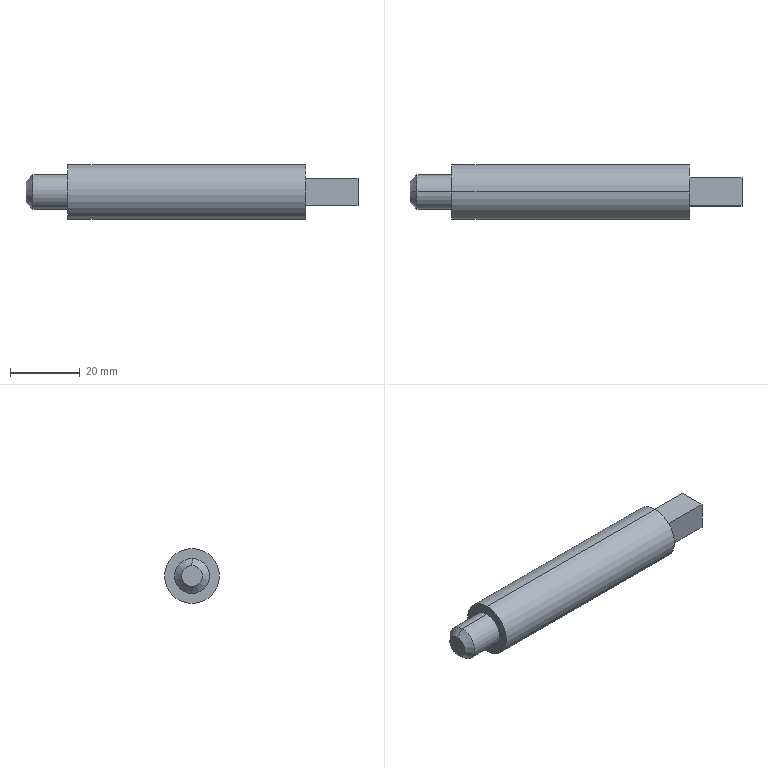Part | SolidWorks | features Chamfer 1, ICE 1, Revolution 1 | 1 solid | 14 faces | box 95 x 15.69 x 15.69 mm | volume 14996 mm3 | plane 8 | cylinder 4 | cone 2 | commonest cylinder face diameters 10 x2 15.69 x2
STEP:
#1=CARTESIAN_POINT('',(0.,0.,3.));
#2=VERTEX_POINT('',#1);
#3=CARTESIAN_POINT('',(0.,0.,-3.));
#4=VERTEX_POINT('',#3);
#5=CARTESIAN_POINT('',(0.,0.,0.));
#6=DIRECTION('',(-1.,0.,0.));
#7=DIRECTION('',(0.,0.,-1.));
#8=AXIS2_PLACEMENT_3D('',#5,#6,#7);
#9=CIRCLE('',#8,3.);
#10=EDGE_CURVE('',#2,#4,#9,.T.);
#11=ORIENTED_EDGE('',*,*,#10,.F.);
#12=CARTESIAN_POINT('',(2.,0.,5.));
#13=VERTEX_POINT('',#12);
#14=CARTESIAN_POINT('',(0.,0.,3.));
#15=DIRECTION('',(0.7071,0.,0.7071));
#16=VECTOR('',#15,1000.);
#17=LINE('',#14,#16);
#18=EDGE_CURVE('',#2,#13,#17,.T.);
#19=ORIENTED_EDGE('',*,*,#18,.T.);
#20=CARTESIAN_POINT('',(2.,0.,-5.));
#21=VERTEX_POINT('',#20);
#22=CARTESIAN_POINT('',(2.,0.,0.));
#23=DIRECTION('',(1.,0.,0.));
#24=DIRECTION('',(0.,0.,-1.));
#25=AXIS2_PLACEMENT_3D('',#22,#23,#24);
#26=CIRCLE('',#25,5.);
#27=EDGE_CURVE('',#21,#13,#26,.T.);
#28=ORIENTED_EDGE('',*,*,#27,.F.);
#29=CARTESIAN_POINT('',(0.,0.,-3.));
#30=DIRECTION('',(0.7071,0.,-0.7071));
#31=VECTOR('',#30,1000.);
#32=LINE('',#29,#31);
#33=EDGE_CURVE('',#4,#21,#32,.T.);
#34=ORIENTED_EDGE('',*,*,#33,.F.);
#35=EDGE_LOOP('',(#11,#19,#28,#34));
#36=FACE_OUTER_BOUND('',#35,.T.);
#37=CARTESIAN_POINT('',(0.,0.,0.));
#38=DIRECTION('',(1.,0.,0.));
#39=DIRECTION('',(0.,0.,-1.));
#40=AXIS2_PLACEMENT_3D('',#37,#38,#39);
#41=CONICAL_SURFACE('',#40,3.,0.7854);
#42=ADVANCED_FACE('',(#36),#41,.T.);
#43=CARTESIAN_POINT('',(80.,0.,7.845));
#44=VERTEX_POINT('',#43);
#45=CARTESIAN_POINT('',(80.,0.,-7.845));
#46=VERTEX_POINT('',#45);
#47=CARTESIAN_POINT('',(80.,0.,0.));
#48=DIRECTION('',(-1.,0.,0.));
#49=DIRECTION('',(0.,0.,1.));
#50=AXIS2_PLACEMENT_3D('',#47,#48,#49);
#51=CIRCLE('',#50,7.845);
#52=EDGE_CURVE('',#44,#46,#51,.T.);
#53=ORIENTED_EDGE('',*,*,#52,.T.);
#54=CARTESIAN_POINT('',(12.,0.,-7.845));
#55=VERTEX_POINT('',#54);
#56=CARTESIAN_POINT('',(0.,0.,-7.845));
#57=DIRECTION('',(-1.,0.,0.));
#58=VECTOR('',#57,1000.);
#59=LINE('',#56,#58);
#60=EDGE_CURVE('',#46,#55,#59,.T.);
#61=ORIENTED_EDGE('',*,*,#60,.T.);
#62=CARTESIAN_POINT('',(12.,0.,7.845));
#63=VERTEX_POINT('',#62);
#64=CARTESIAN_POINT('',(12.,0.,0.));
#65=DIRECTION('',(-1.,0.,0.));
#66=DIRECTION('',(0.,0.,1.));
#67=AXIS2_PLACEMENT_3D('',#64,#65,#66);
#68=CIRCLE('',#67,7.845);
#69=EDGE_CURVE('',#63,#55,#68,.T.);
#70=ORIENTED_EDGE('',*,*,#69,.F.);
#71=CARTESIAN_POINT('',(0.,0.,7.845));
#72=DIRECTION('',(-1.,0.,0.));
#73=VECTOR('',#72,1000.);
#74=LINE('',#71,#73);
#75=EDGE_CURVE('',#44,#63,#74,.T.);
#76=ORIENTED_EDGE('',*,*,#75,.F.);
#77=EDGE_LOOP('',(#53,#61,#70,#76));
#78=FACE_OUTER_BOUND('',#77,.T.);
#79=CARTESIAN_POINT('',(0.,0.,0.));
#80=DIRECTION('',(-1.,0.,0.));
#81=DIRECTION('',(0.,0.,1.));
#82=AXIS2_PLACEMENT_3D('',#79,#80,#81);
#83=CYLINDRICAL_SURFACE('',#82,7.845);
#84=ADVANCED_FACE('',(#78),#83,.T.);
#85=CARTESIAN_POINT('',(12.,0.,5.));
#86=VERTEX_POINT('',#85);
#87=CARTESIAN_POINT('',(12.,0.,-5.));
#88=VERTEX_POINT('',#87);
#89=CARTESIAN_POINT('',(12.,0.,0.));
#90=DIRECTION('',(-1.,0.,0.));
#91=DIRECTION('',(0.,0.,1.));
#92=AXIS2_PLACEMENT_3D('',#89,#90,#91);
#93=CIRCLE('',#92,5.);
#94=EDGE_CURVE('',#86,#88,#93,.T.);
#95=ORIENTED_EDGE('',*,*,#94,.T.);
#96=CARTESIAN_POINT('',(0.,0.,-5.));
#97=DIRECTION('',(-1.,0.,0.));
#98=VECTOR('',#97,1000.);
#99=LINE('',#96,#98);
#100=EDGE_CURVE('',#88,#21,#99,.T.);
#101=ORIENTED_EDGE('',*,*,#100,.T.);
#102=ORIENTED_EDGE('',*,*,#27,.T.);
#103=CARTESIAN_POINT('',(0.,0.,5.));
#104=DIRECTION('',(-1.,0.,0.));
#105=VECTOR('',#104,1000.);
#106=LINE('',#103,#105);
#107=EDGE_CURVE('',#86,#13,#106,.T.);
#108=ORIENTED_EDGE('',*,*,#107,.F.);
#109=EDGE_LOOP('',(#95,#101,#102,#108));
#110=FACE_OUTER_BOUND('',#109,.T.);
#111=CARTESIAN_POINT('',(0.,0.,0.));
#112=DIRECTION('',(-1.,0.,0.));
#113=DIRECTION('',(0.,0.,1.));
#114=AXIS2_PLACEMENT_3D('',#111,#112,#113);
#115=CYLINDRICAL_SURFACE('',#114,5.);
#116=ADVANCED_FACE('',(#110),#115,.T.);
#117=ORIENTED_EDGE('',*,*,#52,.F.);
#118=CARTESIAN_POINT('',(80.,0.,0.));
#119=DIRECTION('',(-1.,0.,0.));
#120=DIRECTION('',(0.,0.,1.));
#121=AXIS2_PLACEMENT_3D('',#118,#119,#120);
#122=CIRCLE('',#121,7.845);
#123=EDGE_CURVE('',#46,#44,#122,.T.);
#124=ORIENTED_EDGE('',*,*,#123,.F.);
#125=EDGE_LOOP('',(#117,#124));
#126=FACE_OUTER_BOUND('',#125,.T.);
#127=CARTESIAN_POINT('',(80.,-4.,-4.));
#128=VERTEX_POINT('',#127);
#129=CARTESIAN_POINT('',(80.,4.,-4.));
#130=VERTEX_POINT('',#129);
#131=CARTESIAN_POINT('',(80.,-4.,-4.));
#132=DIRECTION('',(0.,1.,0.));
#133=VECTOR('',#132,1000.);
#134=LINE('',#131,#133);
#135=EDGE_CURVE('',#128,#130,#134,.T.);
#136=ORIENTED_EDGE('',*,*,#135,.F.);
#137=CARTESIAN_POINT('',(80.,-4.,4.));
#138=VERTEX_POINT('',#137);
#139=CARTESIAN_POINT('',(80.,-4.,4.));
#140=DIRECTION('',(0.,0.,-1.));
#141=VECTOR('',#140,1000.);
#142=LINE('',#139,#141);
#143=EDGE_CURVE('',#138,#128,#142,.T.);
#144=ORIENTED_EDGE('',*,*,#143,.F.);
#145=CARTESIAN_POINT('',(80.,4.,4.));
#146=VERTEX_POINT('',#145);
#147=CARTESIAN_POINT('',(80.,-4.,4.));
#148=DIRECTION('',(0.,-1.,0.));
#149=VECTOR('',#148,1000.);
#150=LINE('',#147,#149);
#151=EDGE_CURVE('',#146,#138,#150,.T.);
#152=ORIENTED_EDGE('',*,*,#151,.F.);
#153=CARTESIAN_POINT('',(80.,4.,4.));
#154=DIRECTION('',(0.,0.,1.));
#155=VECTOR('',#154,1000.);
#156=LINE('',#153,#155);
#157=EDGE_CURVE('',#130,#146,#156,.T.);
#158=ORIENTED_EDGE('',*,*,#157,.F.);
#159=EDGE_LOOP('',(#136,#144,#152,#158));
#160=FACE_BOUND('',#159,.T.);
#161=CARTESIAN_POINT('',(80.,7.845,0.));
#162=DIRECTION('',(-1.,0.,0.));
#163=DIRECTION('',(0.,0.,1.));
#164=AXIS2_PLACEMENT_3D('',#161,#162,#163);
#165=PLANE('',#164);
#166=ADVANCED_FACE('',(#126,#160),#165,.F.);
#167=CARTESIAN_POINT('',(0.,0.,0.));
#168=DIRECTION('',(-1.,0.,0.));
#169=DIRECTION('',(0.,0.,-1.));
#170=AXIS2_PLACEMENT_3D('',#167,#168,#169);
#171=CIRCLE('',#170,3.);
#172=EDGE_CURVE('',#4,#2,#171,.T.);
#173=ORIENTED_EDGE('',*,*,#172,.T.);
#174=ORIENTED_EDGE('',*,*,#10,.T.);
#175=EDGE_LOOP('',(#173,#174));
#176=FACE_OUTER_BOUND('',#175,.T.);
#177=CARTESIAN_POINT('',(0.,0.,0.));
#178=DIRECTION('',(1.,0.,0.));
#179=DIRECTION('',(0.,0.,-1.));
#180=AXIS2_PLACEMENT_3D('',#177,#178,#179);
#181=PLANE('',#180);
#182=ADVANCED_FACE('',(#176),#181,.F.);
#183=ORIENTED_EDGE('',*,*,#100,.F.);
#184=CARTESIAN_POINT('',(12.,0.,0.));
#185=DIRECTION('',(-1.,0.,0.));
#186=DIRECTION('',(0.,0.,1.));
#187=AXIS2_PLACEMENT_3D('',#184,#185,#186);
#188=CIRCLE('',#187,5.);
#189=EDGE_CURVE('',#88,#86,#188,.T.);
#190=ORIENTED_EDGE('',*,*,#189,.T.);
#191=ORIENTED_EDGE('',*,*,#107,.T.);
#192=CARTESIAN_POINT('',(2.,0.,0.));
#193=DIRECTION('',(1.,0.,0.));
#194=DIRECTION('',(0.,0.,-1.));
#195=AXIS2_PLACEMENT_3D('',#192,#193,#194);
#196=CIRCLE('',#195,5.);
#197=EDGE_CURVE('',#13,#21,#196,.T.);
#198=ORIENTED_EDGE('',*,*,#197,.T.);
#199=EDGE_LOOP('',(#183,#190,#191,#198));
#200=FACE_OUTER_BOUND('',#199,.T.);
#201=CARTESIAN_POINT('',(0.,0.,0.));
#202=DIRECTION('',(-1.,0.,0.));
#203=DIRECTION('',(0.,0.,1.));
#204=AXIS2_PLACEMENT_3D('',#201,#202,#203);
#205=CYLINDRICAL_SURFACE('',#204,5.);
#206=ADVANCED_FACE('',(#200),#205,.T.);
#207=ORIENTED_EDGE('',*,*,#94,.F.);
#208=ORIENTED_EDGE('',*,*,#189,.F.);
#209=EDGE_LOOP('',(#207,#208));
#210=FACE_BOUND('',#209,.T.);
#211=ORIENTED_EDGE('',*,*,#69,.T.);
#212=CARTESIAN_POINT('',(12.,0.,0.));
#213=DIRECTION('',(-1.,0.,0.));
#214=DIRECTION('',(0.,0.,1.));
#215=AXIS2_PLACEMENT_3D('',#212,#213,#214);
#216=CIRCLE('',#215,7.845);
#217=EDGE_CURVE('',#55,#63,#216,.T.);
#218=ORIENTED_EDGE('',*,*,#217,.T.);
#219=EDGE_LOOP('',(#211,#218));
#220=FACE_OUTER_BOUND('',#219,.T.);
#221=CARTESIAN_POINT('',(12.,5.,0.));
#222=DIRECTION('',(1.,0.,0.));
#223=DIRECTION('',(0.,0.,-1.));
#224=AXIS2_PLACEMENT_3D('',#221,#222,#223);
#225=PLANE('',#224);
#226=ADVANCED_FACE('',(#210,#220),#225,.F.);
#227=ORIENTED_EDGE('',*,*,#60,.F.);
#228=ORIENTED_EDGE('',*,*,#123,.T.);
#229=ORIENTED_EDGE('',*,*,#75,.T.);
#230=ORIENTED_EDGE('',*,*,#217,.F.);
#231=EDGE_LOOP('',(#227,#228,#229,#230));
#232=FACE_OUTER_BOUND('',#231,.T.);
#233=CARTESIAN_POINT('',(0.,0.,0.));
#234=DIRECTION('',(-1.,0.,0.));
#235=DIRECTION('',(0.,0.,1.));
#236=AXIS2_PLACEMENT_3D('',#233,#234,#235);
#237=CYLINDRICAL_SURFACE('',#236,7.845);
#238=ADVANCED_FACE('',(#232),#237,.T.);
#239=ORIENTED_EDGE('',*,*,#135,.T.);
#240=CARTESIAN_POINT('',(95.,4.,-4.));
#241=VERTEX_POINT('',#240);
#242=CARTESIAN_POINT('',(95.,4.,-4.));
#243=DIRECTION('',(-1.,0.,0.));
#244=VECTOR('',#243,1000.);
#245=LINE('',#242,#244);
#246=EDGE_CURVE('',#241,#130,#245,.T.);
#247=ORIENTED_EDGE('',*,*,#246,.F.);
#248=CARTESIAN_POINT('',(95.,-4.,-4.));
#249=VERTEX_POINT('',#248);
#250=CARTESIAN_POINT('',(95.,-4.,-4.));
#251=DIRECTION('',(0.,1.,0.));
#252=VECTOR('',#251,1000.);
#253=LINE('',#250,#252);
#254=EDGE_CURVE('',#249,#241,#253,.T.);
#255=ORIENTED_EDGE('',*,*,#254,.F.);
#256=CARTESIAN_POINT('',(95.,-4.,-4.));
#257=DIRECTION('',(-1.,0.,0.));
#258=VECTOR('',#257,1000.);
#259=LINE('',#256,#258);
#260=EDGE_CURVE('',#249,#128,#259,.T.);
#261=ORIENTED_EDGE('',*,*,#260,.T.);
#262=EDGE_LOOP('',(#239,#247,#255,#261));
#263=FACE_OUTER_BOUND('',#262,.T.);
#264=CARTESIAN_POINT('',(95.,-4.,-4.));
#265=DIRECTION('',(0.,0.,1.));
#266=DIRECTION('',(1.,0.,0.));
#267=AXIS2_PLACEMENT_3D('',#264,#265,#266);
#268=PLANE('',#267);
#269=ADVANCED_FACE('',(#263),#268,.F.);
#270=ORIENTED_EDGE('',*,*,#157,.T.);
#271=CARTESIAN_POINT('',(95.,4.,4.));
#272=VERTEX_POINT('',#271);
#273=CARTESIAN_POINT('',(95.,4.,4.));
#274=DIRECTION('',(-1.,0.,0.));
#275=VECTOR('',#274,1000.);
#276=LINE('',#273,#275);
#277=EDGE_CURVE('',#272,#146,#276,.T.);
#278=ORIENTED_EDGE('',*,*,#277,.F.);
#279=CARTESIAN_POINT('',(95.,4.,4.));
#280=DIRECTION('',(0.,0.,1.));
#281=VECTOR('',#280,1000.);
#282=LINE('',#279,#281);
#283=EDGE_CURVE('',#241,#272,#282,.T.);
#284=ORIENTED_EDGE('',*,*,#283,.F.);
#285=ORIENTED_EDGE('',*,*,#246,.T.);
#286=EDGE_LOOP('',(#270,#278,#284,#285));
#287=FACE_OUTER_BOUND('',#286,.T.);
#288=CARTESIAN_POINT('',(95.,4.,4.));
#289=DIRECTION('',(0.,-1.,0.));
#290=DIRECTION('',(0.,0.,-1.));
#291=AXIS2_PLACEMENT_3D('',#288,#289,#290);
#292=PLANE('',#291);
#293=ADVANCED_FACE('',(#287),#292,.F.);
#294=ORIENTED_EDGE('',*,*,#151,.T.);
#295=CARTESIAN_POINT('',(95.,-4.,4.));
#296=VERTEX_POINT('',#295);
#297=CARTESIAN_POINT('',(95.,-4.,4.));
#298=DIRECTION('',(-1.,0.,0.));
#299=VECTOR('',#298,1000.);
#300=LINE('',#297,#299);
#301=EDGE_CURVE('',#296,#138,#300,.T.);
#302=ORIENTED_EDGE('',*,*,#301,.F.);
#303=CARTESIAN_POINT('',(95.,-4.,4.));
#304=DIRECTION('',(0.,-1.,0.));
#305=VECTOR('',#304,1000.);
#306=LINE('',#303,#305);
#307=EDGE_CURVE('',#272,#296,#306,.T.);
#308=ORIENTED_EDGE('',*,*,#307,.F.);
#309=ORIENTED_EDGE('',*,*,#277,.T.);
#310=EDGE_LOOP('',(#294,#302,#308,#309));
#311=FACE_OUTER_BOUND('',#310,.T.);
#312=CARTESIAN_POINT('',(95.,-4.,4.));
#313=DIRECTION('',(0.,0.,-1.));
#314=DIRECTION('',(-1.,0.,0.));
#315=AXIS2_PLACEMENT_3D('',#312,#313,#314);
#316=PLANE('',#315);
#317=ADVANCED_FACE('',(#311),#316,.F.);
#318=ORIENTED_EDGE('',*,*,#143,.T.);
#319=ORIENTED_EDGE('',*,*,#260,.F.);
#320=CARTESIAN_POINT('',(95.,-4.,4.));
#321=DIRECTION('',(0.,0.,-1.));
#322=VECTOR('',#321,1000.);
#323=LINE('',#320,#322);
#324=EDGE_CURVE('',#296,#249,#323,.T.);
#325=ORIENTED_EDGE('',*,*,#324,.F.);
#326=ORIENTED_EDGE('',*,*,#301,.T.);
#327=EDGE_LOOP('',(#318,#319,#325,#326));
#328=FACE_OUTER_BOUND('',#327,.T.);
#329=CARTESIAN_POINT('',(95.,-4.,4.));
#330=DIRECTION('',(0.,1.,0.));
#331=DIRECTION('',(0.,0.,1.));
#332=AXIS2_PLACEMENT_3D('',#329,#330,#331);
#333=PLANE('',#332);
#334=ADVANCED_FACE('',(#328),#333,.F.);
#335=ORIENTED_EDGE('',*,*,#254,.T.);
#336=ORIENTED_EDGE('',*,*,#283,.T.);
#337=ORIENTED_EDGE('',*,*,#307,.T.);
#338=ORIENTED_EDGE('',*,*,#324,.T.);
#339=EDGE_LOOP('',(#335,#336,#337,#338));
#340=FACE_OUTER_BOUND('',#339,.T.);
#341=CARTESIAN_POINT('',(95.,0.,0.));
#342=DIRECTION('',(-1.,0.,0.));
#343=DIRECTION('',(0.,0.,1.));
#344=AXIS2_PLACEMENT_3D('',#341,#342,#343);
#345=PLANE('',#344);
#346=ADVANCED_FACE('',(#340),#345,.F.);
#347=ORIENTED_EDGE('',*,*,#18,.F.);
#348=ORIENTED_EDGE('',*,*,#172,.F.);
#349=ORIENTED_EDGE('',*,*,#33,.T.);
#350=ORIENTED_EDGE('',*,*,#197,.F.);
#351=EDGE_LOOP('',(#347,#348,#349,#350));
#352=FACE_OUTER_BOUND('',#351,.T.);
#353=CARTESIAN_POINT('',(0.,0.,0.));
#354=DIRECTION('',(1.,0.,0.));
#355=DIRECTION('',(0.,0.,-1.));
#356=AXIS2_PLACEMENT_3D('',#353,#354,#355);
#357=CONICAL_SURFACE('',#356,3.,0.7854);
#358=ADVANCED_FACE('',(#352),#357,.T.);
#359=CLOSED_SHELL('',(#42,#84,#116,#166,#182,#206,#226,#238,#269,#293,#317,#334,#346,#358));
#360=MANIFOLD_SOLID_BREP('',#359);
#361=CARTESIAN_POINT('',(0.,0.,0.));
#362=DIRECTION('',(0.,0.,1.));
#363=DIRECTION('',(1.,0.,0.));
#364=AXIS2_PLACEMENT_3D('',#361,#362,#363);
#365=(LENGTH_UNIT()NAMED_UNIT(*)SI_UNIT(.MILLI.,.METRE.));
#366=UNCERTAINTY_MEASURE_WITH_UNIT(LENGTH_MEASURE(0.00001),#365,'','');
#367=(NAMED_UNIT(*)PLANE_ANGLE_UNIT()SI_UNIT($,.RADIAN.));
#368=(NAMED_UNIT(*)SI_UNIT($,.STERADIAN.)SOLID_ANGLE_UNIT());
#369=(GEOMETRIC_REPRESENTATION_CONTEXT(3)GLOBAL_UNCERTAINTY_ASSIGNED_CONTEXT((#366))GLOBAL_UNIT_ASSIGNED_CONTEXT((#365,#367,#368))REPRESENTATION_CONTEXT('',''));
#370=ADVANCED_BREP_SHAPE_REPRESENTATION('',(#360,#364),#369);